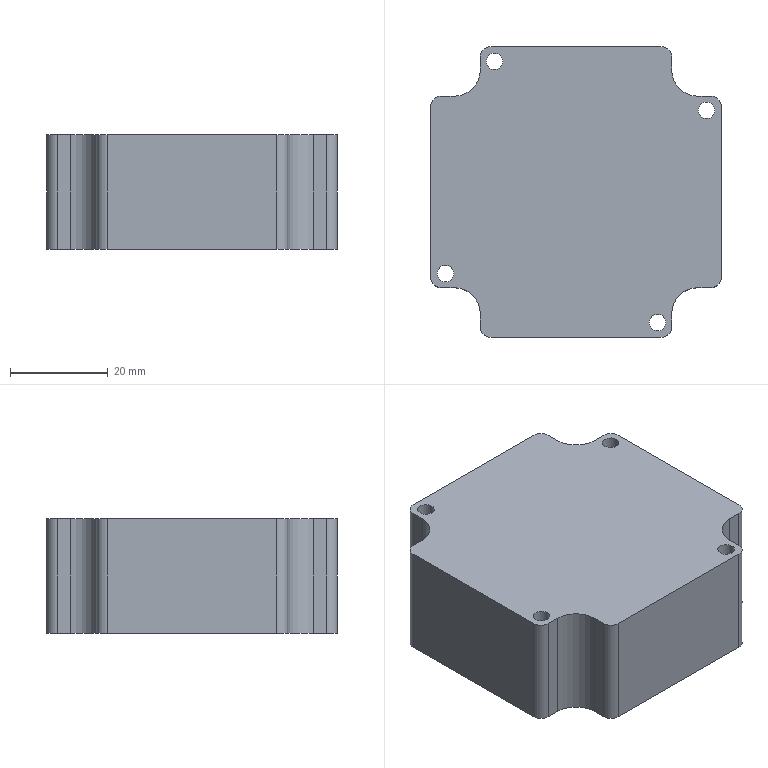Part | STEP file | 1 solid | 34 faces | box 59.4 x 59.4 x 23.3 mm | volume 72108 mm3 | cylinder 18 | plane 16 | commonest cylinder face diameters 4.4 x8 3.4 x4 10.6 x4 3.645 x2